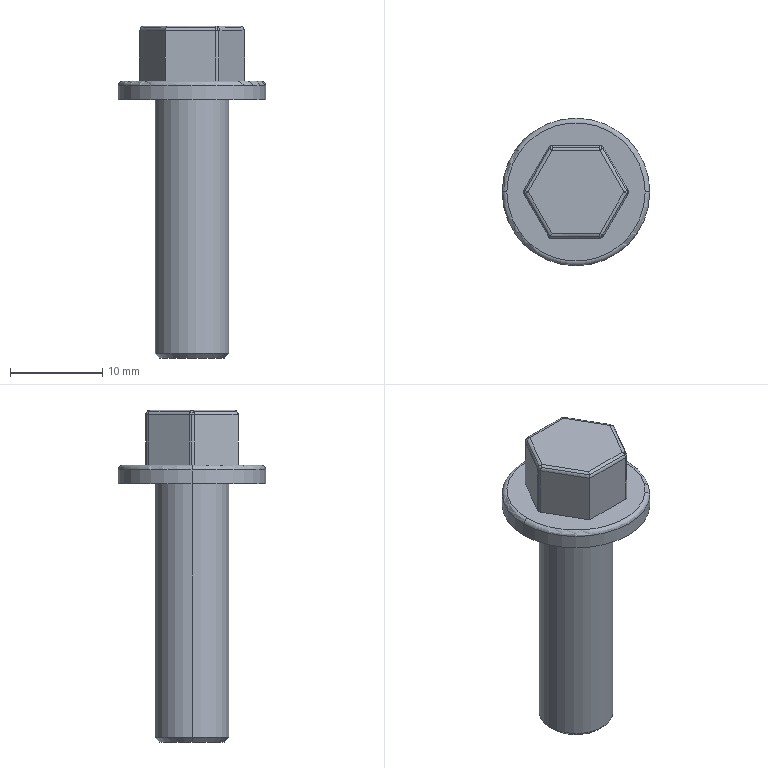Part | SolidWorks | features BaseBody 1 | 1 solid | 50 faces | box 16 x 16 x 36 mm | volume 2321 mm3 | cylinder 26 | sphere 10 | plane 10 | cone 2 | torus 2 | commonest cylinder face diameters 1 x22 8 x2 16 x2
STEP:
#1=CARTESIAN_POINT('',(3.5,0.,-28.));
#2=VERTEX_POINT('',#1);
#3=CARTESIAN_POINT('',(-3.5,0.,-28.));
#4=VERTEX_POINT('',#3);
#5=CARTESIAN_POINT('',(0.,0.,-28.));
#6=DIRECTION('',(0.,0.,1.));
#7=DIRECTION('',(1.,0.,0.));
#8=AXIS2_PLACEMENT_3D('',#5,#6,#7);
#9=CIRCLE('',#8,3.5);
#10=EDGE_CURVE('',#2,#4,#9,.T.);
#11=ORIENTED_EDGE('',*,*,#10,.T.);
#12=CARTESIAN_POINT('',(-4.,0.,-27.5));
#13=VERTEX_POINT('',#12);
#14=CARTESIAN_POINT('',(-3.75,0.,-27.75));
#15=DIRECTION('',(-0.7071,0.,0.7071));
#16=VECTOR('',#15,1000.);
#17=LINE('',#14,#16);
#18=EDGE_CURVE('',#4,#13,#17,.T.);
#19=ORIENTED_EDGE('',*,*,#18,.T.);
#20=CARTESIAN_POINT('',(4.,0.,-27.5));
#21=VERTEX_POINT('',#20);
#22=CARTESIAN_POINT('',(0.,0.,-27.5));
#23=DIRECTION('',(0.,0.,-1.));
#24=DIRECTION('',(1.,0.,0.));
#25=AXIS2_PLACEMENT_3D('',#22,#23,#24);
#26=CIRCLE('',#25,4.);
#27=EDGE_CURVE('',#13,#21,#26,.T.);
#28=ORIENTED_EDGE('',*,*,#27,.T.);
#29=CARTESIAN_POINT('',(3.75,0.,-27.75));
#30=DIRECTION('',(0.7071,0.,0.7071));
#31=VECTOR('',#30,1000.);
#32=LINE('',#29,#31);
#33=EDGE_CURVE('',#2,#21,#32,.T.);
#34=ORIENTED_EDGE('',*,*,#33,.F.);
#35=EDGE_LOOP('',(#11,#19,#28,#34));
#36=FACE_OUTER_BOUND('',#35,.T.);
#37=CARTESIAN_POINT('',(0.,0.,-27.75));
#38=DIRECTION('',(0.,0.,1.));
#39=DIRECTION('',(1.,0.,0.));
#40=AXIS2_PLACEMENT_3D('',#37,#38,#39);
#41=CONICAL_SURFACE('',#40,3.75,0.7854);
#42=ADVANCED_FACE('',(#36),#41,.T.);
#43=ORIENTED_EDGE('',*,*,#27,.F.);
#44=CARTESIAN_POINT('',(-4.,0.,0.));
#45=VERTEX_POINT('',#44);
#46=CARTESIAN_POINT('',(-4.,0.,0.));
#47=DIRECTION('',(0.,0.,1.));
#48=VECTOR('',#47,1000.);
#49=LINE('',#46,#48);
#50=EDGE_CURVE('',#13,#45,#49,.T.);
#51=ORIENTED_EDGE('',*,*,#50,.T.);
#52=CARTESIAN_POINT('',(4.,0.,0.));
#53=VERTEX_POINT('',#52);
#54=CARTESIAN_POINT('',(0.,0.,0.));
#55=DIRECTION('',(0.,0.,1.));
#56=DIRECTION('',(1.,0.,0.));
#57=AXIS2_PLACEMENT_3D('',#54,#55,#56);
#58=CIRCLE('',#57,4.);
#59=EDGE_CURVE('',#53,#45,#58,.T.);
#60=ORIENTED_EDGE('',*,*,#59,.F.);
#61=CARTESIAN_POINT('',(4.,0.,0.));
#62=DIRECTION('',(0.,0.,1.));
#63=VECTOR('',#62,1000.);
#64=LINE('',#61,#63);
#65=EDGE_CURVE('',#21,#53,#64,.T.);
#66=ORIENTED_EDGE('',*,*,#65,.F.);
#67=EDGE_LOOP('',(#43,#51,#60,#66));
#68=FACE_OUTER_BOUND('',#67,.T.);
#69=CARTESIAN_POINT('',(0.,0.,0.));
#70=DIRECTION('',(0.,0.,1.));
#71=DIRECTION('',(1.,0.,0.));
#72=AXIS2_PLACEMENT_3D('',#69,#70,#71);
#73=CYLINDRICAL_SURFACE('',#72,4.);
#74=ADVANCED_FACE('',(#68),#73,.T.);
#75=CARTESIAN_POINT('',(2.784,-4.964,7.5));
#76=VERTEX_POINT('',#75);
#77=CARTESIAN_POINT('',(2.598,-5.,7.5));
#78=VERTEX_POINT('',#77);
#79=CARTESIAN_POINT('',(2.598,-4.5,7.5));
#80=DIRECTION('',(0.,0.,-1.));
#81=DIRECTION('',(0.866,-0.5,0.));
#82=AXIS2_PLACEMENT_3D('',#79,#80,#81);
#83=CIRCLE('',#82,0.5);
#84=EDGE_CURVE('',#76,#78,#83,.T.);
#85=ORIENTED_EDGE('',*,*,#84,.F.);
#86=CARTESIAN_POINT('',(2.759,-4.593,7.964));
#87=VERTEX_POINT('',#86);
#88=CARTESIAN_POINT('',(2.598,-4.5,7.5));
#89=DIRECTION('',(-0.9014,-0.3603,0.2402));
#90=DIRECTION('',(0.3712,-0.9286,0.));
#91=AXIS2_PLACEMENT_3D('',#88,#89,#90);
#92=CIRCLE('',#91,0.5);
#93=EDGE_CURVE('',#76,#87,#92,.T.);
#94=ORIENTED_EDGE('',*,*,#93,.T.);
#95=CARTESIAN_POINT('',(2.598,-4.5,8.));
#96=VERTEX_POINT('',#95);
#97=CARTESIAN_POINT('',(2.598,-4.5,7.5));
#98=DIRECTION('',(0.5,0.866,0.));
#99=DIRECTION('',(0.,0.,1.));
#100=AXIS2_PLACEMENT_3D('',#97,#98,#99);
#101=CIRCLE('',#100,0.5);
#102=EDGE_CURVE('',#96,#87,#101,.T.);
#103=ORIENTED_EDGE('',*,*,#102,.F.);
#104=CARTESIAN_POINT('',(2.598,-4.854,7.854));
#105=VERTEX_POINT('',#104);
#106=CARTESIAN_POINT('',(2.598,-4.5,7.5));
#107=DIRECTION('',(-1.,0.,0.));
#108=DIRECTION('',(0.,-1.,0.));
#109=AXIS2_PLACEMENT_3D('',#106,#107,#108);
#110=CIRCLE('',#109,0.5);
#111=EDGE_CURVE('',#105,#96,#110,.T.);
#112=ORIENTED_EDGE('',*,*,#111,.F.);
#113=CARTESIAN_POINT('',(2.598,-4.5,7.5));
#114=DIRECTION('',(-1.,0.,0.));
#115=DIRECTION('',(0.,-1.,0.));
#116=AXIS2_PLACEMENT_3D('',#113,#114,#115);
#117=CIRCLE('',#116,0.5);
#118=EDGE_CURVE('',#78,#105,#117,.T.);
#119=ORIENTED_EDGE('',*,*,#118,.F.);
#120=EDGE_LOOP('',(#85,#94,#103,#112,#119));
#121=FACE_OUTER_BOUND('',#120,.T.);
#122=CARTESIAN_POINT('',(2.598,-4.5,7.5));
#123=DIRECTION('',(0.9014,0.3603,-0.2402));
#124=DIRECTION('',(0.433,-0.75,0.5));
#125=AXIS2_PLACEMENT_3D('',#122,#123,#124);
#126=SPHERICAL_SURFACE('',#125,0.5);
#127=ADVANCED_FACE('',(#121),#126,.T.);
#128=CARTESIAN_POINT('',(3.031,-4.75,7.5));
#129=VERTEX_POINT('',#128);
#130=CARTESIAN_POINT('',(2.848,-4.933,7.5));
#131=VERTEX_POINT('',#130);
#132=CARTESIAN_POINT('',(2.598,-4.5,7.5));
#133=DIRECTION('',(0.,0.,-1.));
#134=DIRECTION('',(0.866,-0.5,0.));
#135=AXIS2_PLACEMENT_3D('',#132,#133,#134);
#136=CIRCLE('',#135,0.5);
#137=EDGE_CURVE('',#129,#131,#136,.T.);
#138=ORIENTED_EDGE('',*,*,#137,.T.);
#139=CARTESIAN_POINT('',(2.848,-4.933,2.));
#140=VERTEX_POINT('',#139);
#141=CARTESIAN_POINT('',(2.848,-4.933,2.));
#142=DIRECTION('',(0.,0.,-1.));
#143=VECTOR('',#142,1000.);
#144=LINE('',#141,#143);
#145=EDGE_CURVE('',#131,#140,#144,.T.);
#146=ORIENTED_EDGE('',*,*,#145,.T.);
#147=CARTESIAN_POINT('',(3.031,-4.75,2.));
#148=VERTEX_POINT('',#147);
#149=CARTESIAN_POINT('',(2.598,-4.5,2.));
#150=DIRECTION('',(0.,0.,1.));
#151=DIRECTION('',(0.5,-0.866,0.));
#152=AXIS2_PLACEMENT_3D('',#149,#150,#151);
#153=CIRCLE('',#152,0.5);
#154=EDGE_CURVE('',#140,#148,#153,.T.);
#155=ORIENTED_EDGE('',*,*,#154,.T.);
#156=CARTESIAN_POINT('',(3.031,-4.75,2.));
#157=DIRECTION('',(0.,0.,1.));
#158=VECTOR('',#157,1000.);
#159=LINE('',#156,#158);
#160=EDGE_CURVE('',#148,#129,#159,.T.);
#161=ORIENTED_EDGE('',*,*,#160,.T.);
#162=EDGE_LOOP('',(#138,#146,#155,#161));
#163=FACE_OUTER_BOUND('',#162,.T.);
#164=CARTESIAN_POINT('',(2.598,-4.5,2.));
#165=DIRECTION('',(0.,0.,-1.));
#166=DIRECTION('',(0.5,-0.866,0.));
#167=AXIS2_PLACEMENT_3D('',#164,#165,#166);
#168=CYLINDRICAL_SURFACE('',#167,0.5);
#169=ADVANCED_FACE('',(#163),#168,.T.);
#170=ORIENTED_EDGE('',*,*,#118,.T.);
#171=CARTESIAN_POINT('',(-2.802,-4.854,7.854));
#172=VERTEX_POINT('',#171);
#173=CARTESIAN_POINT('',(-1.443,-4.854,7.854));
#174=DIRECTION('',(-1.,0.,0.));
#175=VECTOR('',#174,1000.);
#176=LINE('',#173,#175);
#177=EDGE_CURVE('',#105,#172,#176,.T.);
#178=ORIENTED_EDGE('',*,*,#177,.T.);
#179=CARTESIAN_POINT('',(-2.887,-5.,7.5));
#180=VERTEX_POINT('',#179);
#181=CARTESIAN_POINT('',(-2.802,-4.854,7.854));
#182=CARTESIAN_POINT('',(-2.857,-4.949,7.759));
#183=CARTESIAN_POINT('',(-2.887,-5.,7.634));
#184=CARTESIAN_POINT('',(-2.887,-5.,7.5));
#185=(BOUNDED_CURVE()B_SPLINE_CURVE(3,(#181,#182,#183,#184),.UNSPECIFIED.,.F.,.F.)B_SPLINE_CURVE_WITH_KNOTS((4,4),(5.498,6.283),.UNSPECIFIED.)CURVE()GEOMETRIC_REPRESENTATION_ITEM()RATIONAL_B_SPLINE_CURVE((1.,0.9493,0.9493,1.))REPRESENTATION_ITEM(''));
#186=EDGE_CURVE('',#172,#180,#185,.T.);
#187=ORIENTED_EDGE('',*,*,#186,.T.);
#188=CARTESIAN_POINT('',(-1.443,-5.,7.5));
#189=DIRECTION('',(1.,0.,0.));
#190=VECTOR('',#189,1000.);
#191=LINE('',#188,#190);
#192=EDGE_CURVE('',#180,#78,#191,.T.);
#193=ORIENTED_EDGE('',*,*,#192,.T.);
#194=EDGE_LOOP('',(#170,#178,#187,#193));
#195=FACE_OUTER_BOUND('',#194,.T.);
#196=CARTESIAN_POINT('',(-1.443,-4.5,7.5));
#197=DIRECTION('',(-1.,0.,0.));
#198=DIRECTION('',(0.,-0.7071,0.7071));
#199=AXIS2_PLACEMENT_3D('',#196,#197,#198);
#200=CYLINDRICAL_SURFACE('',#199,0.5);
#201=ADVANCED_FACE('',(#195),#200,.T.);
#202=CARTESIAN_POINT('',(-5.583,-0.2236,7.724));
#203=VERTEX_POINT('',#202);
#204=CARTESIAN_POINT('',(-5.629,-0.25,7.5));
#205=VERTEX_POINT('',#204);
#206=CARTESIAN_POINT('',(-5.196,0.,7.5));
#207=DIRECTION('',(0.5,-0.866,0.));
#208=DIRECTION('',(0.,0.,1.));
#209=AXIS2_PLACEMENT_3D('',#206,#207,#208);
#210=CIRCLE('',#209,0.5);
#211=EDGE_CURVE('',#203,#205,#210,.T.);
#212=ORIENTED_EDGE('',*,*,#211,.F.);
#213=CARTESIAN_POINT('',(-5.583,0.2236,7.724));
#214=VERTEX_POINT('',#213);
#215=CARTESIAN_POINT('',(-5.196,0.,7.5));
#216=DIRECTION('',(-0.5,0.,-0.866));
#217=DIRECTION('',(-0.866,0.,0.5));
#218=AXIS2_PLACEMENT_3D('',#215,#216,#217);
#219=CIRCLE('',#218,0.5);
#220=EDGE_CURVE('',#203,#214,#219,.T.);
#221=ORIENTED_EDGE('',*,*,#220,.T.);
#222=CARTESIAN_POINT('',(-5.629,0.25,7.5));
#223=VERTEX_POINT('',#222);
#224=CARTESIAN_POINT('',(-5.196,0.,7.5));
#225=DIRECTION('',(0.5,0.866,0.));
#226=DIRECTION('',(-0.866,0.5,0.));
#227=AXIS2_PLACEMENT_3D('',#224,#225,#226);
#228=CIRCLE('',#227,0.5);
#229=EDGE_CURVE('',#223,#214,#228,.T.);
#230=ORIENTED_EDGE('',*,*,#229,.F.);
#231=CARTESIAN_POINT('',(-5.696,0.,7.5));
#232=VERTEX_POINT('',#231);
#233=CARTESIAN_POINT('',(-5.196,0.,7.5));
#234=DIRECTION('',(0.,0.,-1.));
#235=DIRECTION('',(-0.866,-0.5,0.));
#236=AXIS2_PLACEMENT_3D('',#233,#234,#235);
#237=CIRCLE('',#236,0.5);
#238=EDGE_CURVE('',#232,#223,#237,.T.);
#239=ORIENTED_EDGE('',*,*,#238,.F.);
#240=CARTESIAN_POINT('',(-5.196,0.,7.5));
#241=DIRECTION('',(0.,0.,-1.));
#242=DIRECTION('',(-0.866,-0.5,0.));
#243=AXIS2_PLACEMENT_3D('',#240,#241,#242);
#244=CIRCLE('',#243,0.5);
#245=EDGE_CURVE('',#205,#232,#244,.T.);
#246=ORIENTED_EDGE('',*,*,#245,.F.);
#247=EDGE_LOOP('',(#212,#221,#230,#239,#246));
#248=FACE_OUTER_BOUND('',#247,.T.);
#249=CARTESIAN_POINT('',(-5.196,0.,7.5));
#250=DIRECTION('',(0.5,0.,0.866));
#251=DIRECTION('',(-0.866,0.,0.5));
#252=AXIS2_PLACEMENT_3D('',#249,#250,#251);
#253=SPHERICAL_SURFACE('',#252,0.5);
#254=ADVANCED_FACE('',(#248),#253,.T.);
#255=ORIENTED_EDGE('',*,*,#245,.T.);
#256=CARTESIAN_POINT('',(-5.696,0.,2.));
#257=VERTEX_POINT('',#256);
#258=CARTESIAN_POINT('',(-5.696,0.,2.));
#259=DIRECTION('',(0.,0.,-1.));
#260=VECTOR('',#259,1000.);
#261=LINE('',#258,#260);
#262=EDGE_CURVE('',#232,#257,#261,.T.);
#263=ORIENTED_EDGE('',*,*,#262,.T.);
#264=CARTESIAN_POINT('',(-5.629,-0.25,2.));
#265=VERTEX_POINT('',#264);
#266=CARTESIAN_POINT('',(-5.196,0.,2.));
#267=DIRECTION('',(0.,0.,1.));
#268=DIRECTION('',(-1.,0.,0.));
#269=AXIS2_PLACEMENT_3D('',#266,#267,#268);
#270=CIRCLE('',#269,0.5);
#271=EDGE_CURVE('',#257,#265,#270,.T.);
#272=ORIENTED_EDGE('',*,*,#271,.T.);
#273=CARTESIAN_POINT('',(-5.629,-0.25,2.));
#274=DIRECTION('',(0.,0.,1.));
#275=VECTOR('',#274,1000.);
#276=LINE('',#273,#275);
#277=EDGE_CURVE('',#265,#205,#276,.T.);
#278=ORIENTED_EDGE('',*,*,#277,.T.);
#279=EDGE_LOOP('',(#255,#263,#272,#278));
#280=FACE_OUTER_BOUND('',#279,.T.);
#281=CARTESIAN_POINT('',(-5.196,0.,2.));
#282=DIRECTION('',(0.,0.,-1.));
#283=DIRECTION('',(-1.,0.,0.));
#284=AXIS2_PLACEMENT_3D('',#281,#282,#283);
#285=CYLINDRICAL_SURFACE('',#284,0.5);
#286=ADVANCED_FACE('',(#280),#285,.T.);
#287=ORIENTED_EDGE('',*,*,#186,.F.);
#288=CARTESIAN_POINT('',(-5.502,-0.1768,7.854));
#289=VERTEX_POINT('',#288);
#290=CARTESIAN_POINT('',(-4.925,-1.177,7.854));
#291=DIRECTION('',(-0.5,0.866,0.));
#292=VECTOR('',#291,1000.);
#293=LINE('',#290,#292);
#294=EDGE_CURVE('',#172,#289,#293,.T.);
#295=ORIENTED_EDGE('',*,*,#294,.T.);
#296=CARTESIAN_POINT('',(-5.196,0.,7.5));
#297=DIRECTION('',(0.5,-0.866,0.));
#298=DIRECTION('',(0.,0.,1.));
#299=AXIS2_PLACEMENT_3D('',#296,#297,#298);
#300=CIRCLE('',#299,0.5);
#301=EDGE_CURVE('',#289,#203,#300,.T.);
#302=ORIENTED_EDGE('',*,*,#301,.T.);
#303=ORIENTED_EDGE('',*,*,#211,.T.);
#304=CARTESIAN_POINT('',(-5.052,-1.25,7.5));
#305=DIRECTION('',(0.5,-0.866,0.));
#306=VECTOR('',#305,1000.);
#307=LINE('',#304,#306);
#308=EDGE_CURVE('',#205,#180,#307,.T.);
#309=ORIENTED_EDGE('',*,*,#308,.T.);
#310=EDGE_LOOP('',(#287,#295,#302,#303,#309));
#311=FACE_OUTER_BOUND('',#310,.T.);
#312=CARTESIAN_POINT('',(-4.619,-1.,7.5));
#313=DIRECTION('',(-0.5,0.866,0.));
#314=DIRECTION('',(-0.6124,-0.3536,0.7071));
#315=AXIS2_PLACEMENT_3D('',#312,#313,#314);
#316=CYLINDRICAL_SURFACE('',#315,0.5);
#317=ADVANCED_FACE('',(#311),#316,.T.);
#318=CARTESIAN_POINT('',(5.583,0.2236,7.724));
#319=VERTEX_POINT('',#318);
#320=CARTESIAN_POINT('',(5.629,0.25,7.5));
#321=VERTEX_POINT('',#320);
#322=CARTESIAN_POINT('',(5.196,0.,7.5));
#323=DIRECTION('',(-0.5,0.866,0.));
#324=DIRECTION('',(0.,0.,1.));
#325=AXIS2_PLACEMENT_3D('',#322,#323,#324);
#326=CIRCLE('',#325,0.5);
#327=EDGE_CURVE('',#319,#321,#326,.T.);
#328=ORIENTED_EDGE('',*,*,#327,.F.);
#329=CARTESIAN_POINT('',(5.583,-0.2236,7.724));
#330=VERTEX_POINT('',#329);
#331=CARTESIAN_POINT('',(5.196,0.,7.5));
#332=DIRECTION('',(0.5,0.,-0.866));
#333=DIRECTION('',(-0.866,0.,-0.5));
#334=AXIS2_PLACEMENT_3D('',#331,#332,#333);
#335=CIRCLE('',#334,0.5);
#336=EDGE_CURVE('',#319,#330,#335,.T.);
#337=ORIENTED_EDGE('',*,*,#336,.T.);
#338=CARTESIAN_POINT('',(5.629,-0.25,7.5));
#339=VERTEX_POINT('',#338);
#340=CARTESIAN_POINT('',(5.196,0.,7.5));
#341=DIRECTION('',(-0.5,-0.866,0.));
#342=DIRECTION('',(0.866,-0.5,0.));
#343=AXIS2_PLACEMENT_3D('',#340,#341,#342);
#344=CIRCLE('',#343,0.5);
#345=EDGE_CURVE('',#339,#330,#344,.T.);
#346=ORIENTED_EDGE('',*,*,#345,.F.);
#347=CARTESIAN_POINT('',(5.696,0.,7.5));
#348=VERTEX_POINT('',#347);
#349=CARTESIAN_POINT('',(5.196,0.,7.5));
#350=DIRECTION('',(0.,0.,-1.));
#351=DIRECTION('',(0.866,0.5,0.));
#352=AXIS2_PLACEMENT_3D('',#349,#350,#351);
#353=CIRCLE('',#352,0.5);
#354=EDGE_CURVE('',#348,#339,#353,.T.);
#355=ORIENTED_EDGE('',*,*,#354,.F.);
#356=CARTESIAN_POINT('',(5.196,0.,7.5));
#357=DIRECTION('',(0.,0.,-1.));
#358=DIRECTION('',(0.866,0.5,0.));
#359=AXIS2_PLACEMENT_3D('',#356,#357,#358);
#360=CIRCLE('',#359,0.5);
#361=EDGE_CURVE('',#321,#348,#360,.T.);
#362=ORIENTED_EDGE('',*,*,#361,.F.);
#363=EDGE_LOOP('',(#328,#337,#346,#355,#362));
#364=FACE_OUTER_BOUND('',#363,.T.);
#365=CARTESIAN_POINT('',(5.196,0.,7.5));
#366=DIRECTION('',(-0.5,0.,0.866));
#367=DIRECTION('',(0.866,0.,0.5));
#368=AXIS2_PLACEMENT_3D('',#365,#366,#367);
#369=SPHERICAL_SURFACE('',#368,0.5);
#370=ADVANCED_FACE('',(#364),#369,.T.);
#371=ORIENTED_EDGE('',*,*,#361,.T.);
#372=CARTESIAN_POINT('',(5.696,0.,2.));
#373=VERTEX_POINT('',#372);
#374=CARTESIAN_POINT('',(5.696,0.,2.));
#375=DIRECTION('',(0.,0.,-1.));
#376=VECTOR('',#375,1000.);
#377=LINE('',#374,#376);
#378=EDGE_CURVE('',#348,#373,#377,.T.);
#379=ORIENTED_EDGE('',*,*,#378,.T.);
#380=CARTESIAN_POINT('',(5.629,0.25,2.));
#381=VERTEX_POINT('',#380);
#382=CARTESIAN_POINT('',(5.196,0.,2.));
#383=DIRECTION('',(0.,0.,1.));
#384=DIRECTION('',(1.,0.,0.));
#385=AXIS2_PLACEMENT_3D('',#382,#383,#384);
#386=CIRCLE('',#385,0.5);
#387=EDGE_CURVE('',#373,#381,#386,.T.);
#388=ORIENTED_EDGE('',*,*,#387,.T.);
#389=CARTESIAN_POINT('',(5.629,0.25,2.));
#390=DIRECTION('',(0.,0.,1.));
#391=VECTOR('',#390,1000.);
#392=LINE('',#389,#391);
#393=EDGE_CURVE('',#381,#321,#392,.T.);
#394=ORIENTED_EDGE('',*,*,#393,.T.);
#395=EDGE_LOOP('',(#371,#379,#388,#394));
#396=FACE_OUTER_BOUND('',#395,.T.);
#397=CARTESIAN_POINT('',(5.196,0.,2.));
#398=DIRECTION('',(0.,0.,-1.));
#399=DIRECTION('',(1.,0.,0.));
#400=AXIS2_PLACEMENT_3D('',#397,#398,#399);
#401=CYLINDRICAL_SURFACE('',#400,0.5);
#402=ADVANCED_FACE('',(#396),#401,.T.);
#403=CARTESIAN_POINT('',(-2.759,4.593,7.964));
#404=VERTEX_POINT('',#403);
#405=CARTESIAN_POINT('',(-2.904,4.677,7.854));
#406=VERTEX_POINT('',#405);
#407=CARTESIAN_POINT('',(-2.598,4.5,7.5));
#408=DIRECTION('',(-0.5,-0.866,0.));
#409=DIRECTION('',(0.,0.,1.));
#410=AXIS2_PLACEMENT_3D('',#407,#408,#409);
#411=CIRCLE('',#410,0.5);
#412=EDGE_CURVE('',#404,#406,#411,.T.);
#413=ORIENTED_EDGE('',*,*,#412,.F.);
#414=CARTESIAN_POINT('',(-2.784,4.964,7.5));
#415=VERTEX_POINT('',#414);
#416=CARTESIAN_POINT('',(-2.598,4.5,7.5));
#417=DIRECTION('',(-0.9014,-0.3603,-0.2402));
#418=DIRECTION('',(0.3712,-0.9286,0.));
#419=AXIS2_PLACEMENT_3D('',#416,#417,#418);
#420=CIRCLE('',#419,0.5);
#421=EDGE_CURVE('',#404,#415,#420,.T.);
#422=ORIENTED_EDGE('',*,*,#421,.T.);
#423=CARTESIAN_POINT('',(-2.848,4.933,7.5));
#424=VERTEX_POINT('',#423);
#425=CARTESIAN_POINT('',(-2.598,4.5,7.5));
#426=DIRECTION('',(0.,0.,-1.));
#427=DIRECTION('',(-0.866,0.5,0.));
#428=AXIS2_PLACEMENT_3D('',#425,#426,#427);
#429=CIRCLE('',#428,0.5);
#430=EDGE_CURVE('',#424,#415,#429,.T.);
#431=ORIENTED_EDGE('',*,*,#430,.F.);
#432=CARTESIAN_POINT('',(-3.031,4.75,7.5));
#433=VERTEX_POINT('',#432);
#434=CARTESIAN_POINT('',(-2.598,4.5,7.5));
#435=DIRECTION('',(0.,0.,-1.));
#436=DIRECTION('',(-0.866,0.5,0.));
#437=AXIS2_PLACEMENT_3D('',#434,#435,#436);
#438=CIRCLE('',#437,0.5);
#439=EDGE_CURVE('',#433,#424,#438,.T.);
#440=ORIENTED_EDGE('',*,*,#439,.F.);
#441=CARTESIAN_POINT('',(-2.598,4.5,7.5));
#442=DIRECTION('',(-0.5,-0.866,0.));
#443=DIRECTION('',(0.,0.,1.));
#444=AXIS2_PLACEMENT_3D('',#441,#442,#443);
#445=CIRCLE('',#444,0.5);
#446=EDGE_CURVE('',#406,#433,#445,.T.);
#447=ORIENTED_EDGE('',*,*,#446,.F.);
#448=EDGE_LOOP('',(#413,#422,#431,#440,#447));
#449=FACE_OUTER_BOUND('',#448,.T.);
#450=CARTESIAN_POINT('',(-2.598,4.5,7.5));
#451=DIRECTION('',(0.9014,0.3603,0.2402));
#452=DIRECTION('',(-0.433,0.75,0.5));
#453=AXIS2_PLACEMENT_3D('',#450,#451,#452);
#454=SPHERICAL_SURFACE('',#453,0.5);
#455=ADVANCED_FACE('',(#449),#454,.T.);
#456=ORIENTED_EDGE('',*,*,#439,.T.);
#457=CARTESIAN_POINT('',(-2.848,4.933,2.));
#458=VERTEX_POINT('',#457);
#459=CARTESIAN_POINT('',(-2.848,4.933,2.));
#460=DIRECTION('',(0.,0.,-1.));
#461=VECTOR('',#460,1000.);
#462=LINE('',#459,#461);
#463=EDGE_CURVE('',#424,#458,#462,.T.);
#464=ORIENTED_EDGE('',*,*,#463,.T.);
#465=CARTESIAN_POINT('',(-3.031,4.75,2.));
#466=VERTEX_POINT('',#465);
#467=CARTESIAN_POINT('',(-2.598,4.5,2.));
#468=DIRECTION('',(0.,0.,1.));
#469=DIRECTION('',(-0.5,0.866,0.));
#470=AXIS2_PLACEMENT_3D('',#467,#468,#469);
#471=CIRCLE('',#470,0.5);
#472=EDGE_CURVE('',#458,#466,#471,.T.);
#473=ORIENTED_EDGE('',*,*,#472,.T.);
#474=CARTESIAN_POINT('',(-3.031,4.75,2.));
#475=DIRECTION('',(0.,0.,1.));
#476=VECTOR('',#475,1000.);
#477=LINE('',#474,#476);
#478=EDGE_CURVE('',#466,#433,#477,.T.);
#479=ORIENTED_EDGE('',*,*,#478,.T.);
#480=EDGE_LOOP('',(#456,#464,#473,#479));
#481=FACE_OUTER_BOUND('',#480,.T.);
#482=CARTESIAN_POINT('',(-2.598,4.5,2.));
#483=DIRECTION('',(0.,0.,-1.));
#484=DIRECTION('',(-0.5,0.866,0.));
#485=AXIS2_PLACEMENT_3D('',#482,#483,#484);
#486=CYLINDRICAL_SURFACE('',#485,0.5);
#487=ADVANCED_FACE('',(#481),#486,.T.);
#488=ORIENTED_EDGE('',*,*,#229,.T.);
#489=CARTESIAN_POINT('',(-5.502,0.1768,7.854));
#490=VERTEX_POINT('',#489);
#491=CARTESIAN_POINT('',(-5.196,0.,7.5));
#492=DIRECTION('',(0.5,0.866,0.));
#493=DIRECTION('',(-0.866,0.5,0.));
#494=AXIS2_PLACEMENT_3D('',#491,#492,#493);
#495=CIRCLE('',#494,0.5);
#496=EDGE_CURVE('',#214,#490,#495,.T.);
#497=ORIENTED_EDGE('',*,*,#496,.T.);
#498=CARTESIAN_POINT('',(-3.482,3.677,7.854));
#499=DIRECTION('',(0.5,0.866,0.));
#500=VECTOR('',#499,1000.);
#501=LINE('',#498,#500);
#502=EDGE_CURVE('',#490,#406,#501,.T.);
#503=ORIENTED_EDGE('',*,*,#502,.T.);
#504=ORIENTED_EDGE('',*,*,#446,.T.);
#505=CARTESIAN_POINT('',(-3.608,3.75,7.5));
#506=DIRECTION('',(-0.5,-0.866,0.));
#507=VECTOR('',#506,1000.);
#508=LINE('',#505,#507);
#509=EDGE_CURVE('',#433,#223,#508,.T.);
#510=ORIENTED_EDGE('',*,*,#509,.T.);
#511=EDGE_LOOP('',(#488,#497,#503,#504,#510));
#512=FACE_OUTER_BOUND('',#511,.T.);
#513=CARTESIAN_POINT('',(-3.175,3.5,7.5));
#514=DIRECTION('',(0.5,0.866,0.));
#515=DIRECTION('',(-0.6124,0.3536,0.7071));
#516=AXIS2_PLACEMENT_3D('',#513,#514,#515);
#517=CYLINDRICAL_SURFACE('',#516,0.5);
#518=ADVANCED_FACE('',(#512),#517,.T.);
#519=CARTESIAN_POINT('',(2.759,4.593,7.964));
#520=VERTEX_POINT('',#519);
#521=CARTESIAN_POINT('',(2.598,4.5,8.));
#522=VERTEX_POINT('',#521);
#523=CARTESIAN_POINT('',(2.598,4.5,7.5));
#524=DIRECTION('',(0.5,-0.866,0.));
#525=DIRECTION('',(0.866,0.5,0.));
#526=AXIS2_PLACEMENT_3D('',#523,#524,#525);
#527=CIRCLE('',#526,0.5);
#528=EDGE_CURVE('',#520,#522,#527,.T.);
#529=ORIENTED_EDGE('',*,*,#528,.F.);
#530=CARTESIAN_POINT('',(2.784,4.964,7.5));
#531=VERTEX_POINT('',#530);
#532=CARTESIAN_POINT('',(2.598,4.5,7.5));
#533=DIRECTION('',(-0.9014,0.3603,0.2402));
#534=DIRECTION('',(-0.3712,-0.9286,0.));
#535=AXIS2_PLACEMENT_3D('',#532,#533,#534);
#536=CIRCLE('',#535,0.5);
#537=EDGE_CURVE('',#520,#531,#536,.T.);
#538=ORIENTED_EDGE('',*,*,#537,.T.);
#539=CARTESIAN_POINT('',(2.598,5.,7.5));
#540=VERTEX_POINT('',#539);
#541=CARTESIAN_POINT('',(2.598,4.5,7.5));
#542=DIRECTION('',(0.,0.,-1.));
#543=DIRECTION('',(0.,1.,0.));
#544=AXIS2_PLACEMENT_3D('',#541,#542,#543);
#545=CIRCLE('',#544,0.5);
#546=EDGE_CURVE('',#540,#531,#545,.T.);
#547=ORIENTED_EDGE('',*,*,#546,.F.);
#548=CARTESIAN_POINT('',(2.598,4.854,7.854));
#549=VERTEX_POINT('',#548);
#550=CARTESIAN_POINT('',(2.598,4.5,7.5));
#551=DIRECTION('',(-1.,0.,0.));
#552=DIRECTION('',(0.,0.,1.));
#553=AXIS2_PLACEMENT_3D('',#550,#551,#552);
#554=CIRCLE('',#553,0.5);
#555=EDGE_CURVE('',#549,#540,#554,.T.);
#556=ORIENTED_EDGE('',*,*,#555,.F.);
#557=CARTESIAN_POINT('',(2.598,4.5,7.5));
#558=DIRECTION('',(-1.,0.,0.));
#559=DIRECTION('',(0.,0.,1.));
#560=AXIS2_PLACEMENT_3D('',#557,#558,#559);
#561=CIRCLE('',#560,0.5);
#562=EDGE_CURVE('',#522,#549,#561,.T.);
#563=ORIENTED_EDGE('',*,*,#562,.F.);
#564=EDGE_LOOP('',(#529,#538,#547,#556,#563));
#565=FACE_OUTER_BOUND('',#564,.T.);
#566=CARTESIAN_POINT('',(2.598,4.5,7.5));
#567=DIRECTION('',(0.9014,-0.3603,-0.2402));
#568=DIRECTION('',(0.433,0.75,0.5));
#569=AXIS2_PLACEMENT_3D('',#566,#567,#568);
#570=SPHERICAL_SURFACE('',#569,0.5);
#571=ADVANCED_FACE('',(#565),#570,.T.);
#572=ORIENTED_EDGE('',*,*,#546,.T.);
#573=CARTESIAN_POINT('',(2.848,4.933,7.5));
#574=VERTEX_POINT('',#573);
#575=CARTESIAN_POINT('',(2.598,4.5,7.5));
#576=DIRECTION('',(0.,0.,-1.));
#577=DIRECTION('',(0.,1.,0.));
#578=AXIS2_PLACEMENT_3D('',#575,#576,#577);
#579=CIRCLE('',#578,0.5);
#580=EDGE_CURVE('',#531,#574,#579,.T.);
#581=ORIENTED_EDGE('',*,*,#580,.T.);
#582=CARTESIAN_POINT('',(2.848,4.933,2.));
#583=VERTEX_POINT('',#582);
#584=CARTESIAN_POINT('',(2.848,4.933,2.));
#585=DIRECTION('',(0.,0.,-1.));
#586=VECTOR('',#585,1000.);
#587=LINE('',#584,#586);
#588=EDGE_CURVE('',#574,#583,#587,.T.);
#589=ORIENTED_EDGE('',*,*,#588,.T.);
#590=CARTESIAN_POINT('',(2.598,5.,2.));
#591=VERTEX_POINT('',#590);
#592=CARTESIAN_POINT('',(2.598,4.5,2.));
#593=DIRECTION('',(0.,0.,1.));
#594=DIRECTION('',(0.5,0.866,0.));
#595=AXIS2_PLACEMENT_3D('',#592,#593,#594);
#596=CIRCLE('',#595,0.5);
#597=EDGE_CURVE('',#583,#591,#596,.T.);
#598=ORIENTED_EDGE('',*,*,#597,.T.);
#599=CARTESIAN_POINT('',(2.598,5.,2.));
#600=DIRECTION('',(0.,0.,1.));
#601=VECTOR('',#600,1000.);
#602=LINE('',#599,#601);
#603=EDGE_CURVE('',#591,#540,#602,.T.);
#604=ORIENTED_EDGE('',*,*,#603,.T.);
#605=EDGE_LOOP('',(#572,#581,#589,#598,#604));
#606=FACE_OUTER_BOUND('',#605,.T.);
#607=CARTESIAN_POINT('',(2.598,4.5,2.));
#608=DIRECTION('',(0.,0.,-1.));
#609=DIRECTION('',(0.5,0.866,0.));
#610=AXIS2_PLACEMENT_3D('',#607,#608,#609);
#611=CYLINDRICAL_SURFACE('',#610,0.5);
#612=ADVANCED_FACE('',(#606),#611,.T.);
#613=CARTESIAN_POINT('',(-2.598,5.,7.5));
#614=VERTEX_POINT('',#613);
#615=CARTESIAN_POINT('',(-2.598,4.854,7.854));
#616=VERTEX_POINT('',#615);
#617=CARTESIAN_POINT('',(-2.598,4.5,7.5));
#618=DIRECTION('',(1.,0.,0.));
#619=DIRECTION('',(0.,1.,0.));
#620=AXIS2_PLACEMENT_3D('',#617,#618,#619);
#621=CIRCLE('',#620,0.5);
#622=EDGE_CURVE('',#614,#616,#621,.T.);
#623=ORIENTED_EDGE('',*,*,#622,.T.);
#624=CARTESIAN_POINT('',(1.443,4.854,7.854));
#625=DIRECTION('',(1.,0.,0.));
#626=VECTOR('',#625,1000.);
#627=LINE('',#624,#626);
#628=EDGE_CURVE('',#616,#549,#627,.T.);
#629=ORIENTED_EDGE('',*,*,#628,.T.);
#630=ORIENTED_EDGE('',*,*,#555,.T.);
#631=CARTESIAN_POINT('',(1.443,5.,7.5));
#632=DIRECTION('',(-1.,0.,0.));
#633=VECTOR('',#632,1000.);
#634=LINE('',#631,#633);
#635=EDGE_CURVE('',#540,#614,#634,.T.);
#636=ORIENTED_EDGE('',*,*,#635,.T.);
#637=EDGE_LOOP('',(#623,#629,#630,#636));
#638=FACE_OUTER_BOUND('',#637,.T.);
#639=CARTESIAN_POINT('',(1.443,4.5,7.5));
#640=DIRECTION('',(1.,0.,0.));
#641=DIRECTION('',(0.,0.7071,0.7071));
#642=AXIS2_PLACEMENT_3D('',#639,#640,#641);
#643=CYLINDRICAL_SURFACE('',#642,0.5);
#644=ADVANCED_FACE('',(#638),#643,.T.);
#645=CARTESIAN_POINT('',(3.031,4.75,7.5));
#646=VERTEX_POINT('',#645);
#647=CARTESIAN_POINT('',(2.904,4.677,7.854));
#648=VERTEX_POINT('',#647);
#649=CARTESIAN_POINT('',(2.598,4.5,7.5));
#650=DIRECTION('',(0.5,-0.866,0.));
#651=DIRECTION('',(0.866,0.5,0.));
#652=AXIS2_PLACEMENT_3D('',#649,#650,#651);
#653=CIRCLE('',#652,0.5);
#654=EDGE_CURVE('',#646,#648,#653,.T.);
#655=ORIENTED_EDGE('',*,*,#654,.T.);
#656=CARTESIAN_POINT('',(5.502,0.1768,7.854));
#657=VERTEX_POINT('',#656);
#658=CARTESIAN_POINT('',(4.925,1.177,7.854));
#659=DIRECTION('',(0.5,-0.866,0.));
#660=VECTOR('',#659,1000.);
#661=LINE('',#658,#660);
#662=EDGE_CURVE('',#648,#657,#661,.T.);
#663=ORIENTED_EDGE('',*,*,#662,.T.);
#664=CARTESIAN_POINT('',(5.196,0.,7.5));
#665=DIRECTION('',(-0.5,0.866,0.));
#666=DIRECTION('',(0.,0.,1.));
#667=AXIS2_PLACEMENT_3D('',#664,#665,#666);
#668=CIRCLE('',#667,0.5);
#669=EDGE_CURVE('',#657,#319,#668,.T.);
#670=ORIENTED_EDGE('',*,*,#669,.T.);
#671=ORIENTED_EDGE('',*,*,#327,.T.);
#672=CARTESIAN_POINT('',(5.052,1.25,7.5));
#673=DIRECTION('',(-0.5,0.866,0.));
#674=VECTOR('',#673,1000.);
#675=LINE('',#672,#674);
#676=EDGE_CURVE('',#321,#646,#675,.T.);
#677=ORIENTED_EDGE('',*,*,#676,.T.);
#678=EDGE_LOOP('',(#655,#663,#670,#671,#677));
#679=FACE_OUTER_BOUND('',#678,.T.);
#680=CARTESIAN_POINT('',(4.619,1.,7.5));
#681=DIRECTION('',(0.5,-0.866,0.));
#682=DIRECTION('',(0.6124,0.3536,0.7071));
#683=AXIS2_PLACEMENT_3D('',#680,#681,#682);
#684=CYLINDRICAL_SURFACE('',#683,0.5);
#685=ADVANCED_FACE('',(#679),#684,.T.);
#686=ORIENTED_EDGE('',*,*,#345,.T.);
#687=CARTESIAN_POINT('',(5.502,-0.1768,7.854));
#688=VERTEX_POINT('',#687);
#689=CARTESIAN_POINT('',(5.196,0.,7.5));
#690=DIRECTION('',(-0.5,-0.866,0.));
#691=DIRECTION('',(0.866,-0.5,0.));
#692=AXIS2_PLACEMENT_3D('',#689,#690,#691);
#693=CIRCLE('',#692,0.5);
#694=EDGE_CURVE('',#330,#688,#693,.T.);
#695=ORIENTED_EDGE('',*,*,#694,.T.);
#696=CARTESIAN_POINT('',(2.904,-4.677,7.854));
#697=VERTEX_POINT('',#696);
#698=CARTESIAN_POINT('',(3.482,-3.677,7.854));
#699=DIRECTION('',(-0.5,-0.866,0.));
#700=VECTOR('',#699,1000.);
#701=LINE('',#698,#700);
#702=EDGE_CURVE('',#688,#697,#701,.T.);
#703=ORIENTED_EDGE('',*,*,#702,.T.);
#704=CARTESIAN_POINT('',(2.598,-4.5,7.5));
#705=DIRECTION('',(0.5,0.866,0.));
#706=DIRECTION('',(0.,0.,1.));
#707=AXIS2_PLACEMENT_3D('',#704,#705,#706);
#708=CIRCLE('',#707,0.5);
#709=EDGE_CURVE('',#697,#129,#708,.T.);
#710=ORIENTED_EDGE('',*,*,#709,.T.);
#711=CARTESIAN_POINT('',(3.608,-3.75,7.5));
#712=DIRECTION('',(0.5,0.866,0.));
#713=VECTOR('',#712,1000.);
#714=LINE('',#711,#713);
#715=EDGE_CURVE('',#129,#339,#714,.T.);
#716=ORIENTED_EDGE('',*,*,#715,.T.);
#717=EDGE_LOOP('',(#686,#695,#703,#710,#716));
#718=FACE_OUTER_BOUND('',#717,.T.);
#719=CARTESIAN_POINT('',(3.175,-3.5,7.5));
#720=DIRECTION('',(-0.5,-0.866,0.));
#721=DIRECTION('',(0.6124,-0.3536,0.7071));
#722=AXIS2_PLACEMENT_3D('',#719,#720,#721);
#723=CYLINDRICAL_SURFACE('',#722,0.5);
#724=ADVANCED_FACE('',(#718),#723,.T.);
#725=CARTESIAN_POINT('',(8.,0.,1.5));
#726=VERTEX_POINT('',#725);
#727=CARTESIAN_POINT('',(-8.,0.,1.5));
#728=VERTEX_POINT('',#727);
#729=CARTESIAN_POINT('',(0.,0.,1.5));
#730=DIRECTION('',(0.,0.,1.));
#731=DIRECTION('',(-1.,0.,0.));
#732=AXIS2_PLACEMENT_3D('',#729,#730,#731);
#733=CIRCLE('',#732,8.);
#734=EDGE_CURVE('',#726,#728,#733,.T.);
#735=ORIENTED_EDGE('',*,*,#734,.T.);
#736=CARTESIAN_POINT('',(-7.5,0.,2.));
#737=VERTEX_POINT('',#736);
#738=CARTESIAN_POINT('',(-7.5,0.,1.5));
#739=DIRECTION('',(0.,1.,0.));
#740=DIRECTION('',(-1.,0.,0.));
#741=AXIS2_PLACEMENT_3D('',#738,#739,#740);
#742=CIRCLE('',#741,0.5);
#743=EDGE_CURVE('',#728,#737,#742,.T.);
#744=ORIENTED_EDGE('',*,*,#743,.T.);
#745=CARTESIAN_POINT('',(7.5,0.,2.));
#746=VERTEX_POINT('',#745);
#747=CARTESIAN_POINT('',(0.,0.,2.));
#748=DIRECTION('',(0.,0.,-1.));
#749=DIRECTION('',(-1.,0.,0.));
#750=AXIS2_PLACEMENT_3D('',#747,#748,#749);
#751=CIRCLE('',#750,7.5);
#752=EDGE_CURVE('',#737,#746,#751,.T.);
#753=ORIENTED_EDGE('',*,*,#752,.T.);
#754=CARTESIAN_POINT('',(7.5,0.,1.5));
#755=DIRECTION('',(0.,-1.,0.));
#756=DIRECTION('',(0.,0.,-1.));
#757=AXIS2_PLACEMENT_3D('',#754,#755,#756);
#758=CIRCLE('',#757,0.5);
#759=EDGE_CURVE('',#726,#746,#758,.T.);
#760=ORIENTED_EDGE('',*,*,#759,.F.);
#761=EDGE_LOOP('',(#735,#744,#753,#760));
#762=FACE_OUTER_BOUND('',#761,.T.);
#763=CARTESIAN_POINT('',(0.,0.,1.5));
#764=DIRECTION('',(0.,0.,1.));
#765=DIRECTION('',(1.,0.,0.));
#766=AXIS2_PLACEMENT_3D('',#763,#764,#765);
#767=TOROIDAL_SURFACE('',#766,7.5,0.5);
#768=ADVANCED_FACE('',(#762),#767,.T.);
#769=ORIENTED_EDGE('',*,*,#734,.F.);
#770=CARTESIAN_POINT('',(8.,0.,0.));
#771=VERTEX_POINT('',#770);
#772=CARTESIAN_POINT('',(8.,0.,0.));
#773=DIRECTION('',(0.,0.,-1.));
#774=VECTOR('',#773,1000.);
#775=LINE('',#772,#774);
#776=EDGE_CURVE('',#726,#771,#775,.T.);
#777=ORIENTED_EDGE('',*,*,#776,.T.);
#778=CARTESIAN_POINT('',(-8.,0.,0.));
#779=VERTEX_POINT('',#778);
#780=CARTESIAN_POINT('',(0.,0.,0.));
#781=DIRECTION('',(0.,0.,-1.));
#782=DIRECTION('',(-1.,0.,0.));
#783=AXIS2_PLACEMENT_3D('',#780,#781,#782);
#784=CIRCLE('',#783,8.);
#785=EDGE_CURVE('',#779,#771,#784,.T.);
#786=ORIENTED_EDGE('',*,*,#785,.F.);
#787=CARTESIAN_POINT('',(-8.,0.,0.));
#788=DIRECTION('',(0.,0.,-1.));
#789=VECTOR('',#788,1000.);
#790=LINE('',#787,#789);
#791=EDGE_CURVE('',#728,#779,#790,.T.);
#792=ORIENTED_EDGE('',*,*,#791,.F.);
#793=EDGE_LOOP('',(#769,#777,#786,#792));
#794=FACE_OUTER_BOUND('',#793,.T.);
#795=CARTESIAN_POINT('',(0.,0.,0.));
#796=DIRECTION('',(0.,0.,-1.));
#797=DIRECTION('',(-1.,0.,0.));
#798=AXIS2_PLACEMENT_3D('',#795,#796,#797);
#799=CYLINDRICAL_SURFACE('',#798,8.);
#800=ADVANCED_FACE('',(#794),#799,.T.);
#801=ORIENTED_EDGE('',*,*,#10,.F.);
#802=CARTESIAN_POINT('',(0.,0.,-28.));
#803=DIRECTION('',(0.,0.,1.));
#804=DIRECTION('',(1.,0.,0.));
#805=AXIS2_PLACEMENT_3D('',#802,#803,#804);
#806=CIRCLE('',#805,3.5);
#807=EDGE_CURVE('',#4,#2,#806,.T.);
#808=ORIENTED_EDGE('',*,*,#807,.F.);
#809=EDGE_LOOP('',(#801,#808));
#810=FACE_OUTER_BOUND('',#809,.T.);
#811=CARTESIAN_POINT('',(0.,0.,-28.));
#812=DIRECTION('',(0.,0.,1.));
#813=DIRECTION('',(1.,0.,0.));
#814=AXIS2_PLACEMENT_3D('',#811,#812,#813);
#815=PLANE('',#814);
#816=ADVANCED_FACE('',(#810),#815,.F.);
#817=ORIENTED_EDGE('',*,*,#308,.F.);
#818=ORIENTED_EDGE('',*,*,#277,.F.);
#819=CARTESIAN_POINT('',(-2.887,-5.,2.));
#820=VERTEX_POINT('',#819);
#821=CARTESIAN_POINT('',(-5.052,-1.25,2.));
#822=DIRECTION('',(-0.5,0.866,0.));
#823=VECTOR('',#822,1000.);
#824=LINE('',#821,#823);
#825=EDGE_CURVE('',#820,#265,#824,.T.);
#826=ORIENTED_EDGE('',*,*,#825,.F.);
#827=CARTESIAN_POINT('',(-2.887,-5.,2.));
#828=DIRECTION('',(0.,0.,1.));
#829=VECTOR('',#828,1000.);
#830=LINE('',#827,#829);
#831=EDGE_CURVE('',#820,#180,#830,.T.);
#832=ORIENTED_EDGE('',*,*,#831,.T.);
#833=EDGE_LOOP('',(#817,#818,#826,#832));
#834=FACE_OUTER_BOUND('',#833,.T.);
#835=CARTESIAN_POINT('',(-5.774,0.,2.));
#836=DIRECTION('',(-0.866,-0.5,0.));
#837=DIRECTION('',(-0.5,0.866,0.));
#838=AXIS2_PLACEMENT_3D('',#835,#836,#837);
#839=PLANE('',#838);
#840=ADVANCED_FACE('',(#834),#839,.T.);
#841=CARTESIAN_POINT('',(-5.629,0.25,2.));
#842=VERTEX_POINT('',#841);
#843=CARTESIAN_POINT('',(-5.629,0.25,2.));
#844=DIRECTION('',(0.,0.,-1.));
#845=VECTOR('',#844,1000.);
#846=LINE('',#843,#845);
#847=EDGE_CURVE('',#223,#842,#846,.T.);
#848=ORIENTED_EDGE('',*,*,#847,.F.);
#849=ORIENTED_EDGE('',*,*,#509,.F.);
#850=ORIENTED_EDGE('',*,*,#478,.F.);
#851=CARTESIAN_POINT('',(-3.608,3.75,2.));
#852=DIRECTION('',(0.5,0.866,0.));
#853=VECTOR('',#852,1000.);
#854=LINE('',#851,#853);
#855=EDGE_CURVE('',#842,#466,#854,.T.);
#856=ORIENTED_EDGE('',*,*,#855,.F.);
#857=EDGE_LOOP('',(#848,#849,#850,#856));
#858=FACE_OUTER_BOUND('',#857,.T.);
#859=CARTESIAN_POINT('',(-2.887,5.,2.));
#860=DIRECTION('',(-0.866,0.5,0.));
#861=DIRECTION('',(0.,0.,1.));
#862=AXIS2_PLACEMENT_3D('',#859,#860,#861);
#863=PLANE('',#862);
#864=ADVANCED_FACE('',(#858),#863,.T.);
#865=CARTESIAN_POINT('',(-2.598,5.,2.));
#866=VERTEX_POINT('',#865);
#867=CARTESIAN_POINT('',(-2.598,5.,2.));
#868=DIRECTION('',(0.,0.,-1.));
#869=VECTOR('',#868,1000.);
#870=LINE('',#867,#869);
#871=EDGE_CURVE('',#614,#866,#870,.T.);
#872=ORIENTED_EDGE('',*,*,#871,.F.);
#873=ORIENTED_EDGE('',*,*,#635,.F.);
#874=ORIENTED_EDGE('',*,*,#603,.F.);
#875=CARTESIAN_POINT('',(1.443,5.,2.));
#876=DIRECTION('',(1.,0.,0.));
#877=VECTOR('',#876,1000.);
#878=LINE('',#875,#877);
#879=EDGE_CURVE('',#866,#591,#878,.T.);
#880=ORIENTED_EDGE('',*,*,#879,.F.);
#881=EDGE_LOOP('',(#872,#873,#874,#880));
#882=FACE_OUTER_BOUND('',#881,.T.);
#883=CARTESIAN_POINT('',(2.887,5.,2.));
#884=DIRECTION('',(0.,1.,0.));
#885=DIRECTION('',(1.,0.,0.));
#886=AXIS2_PLACEMENT_3D('',#883,#884,#885);
#887=PLANE('',#886);
#888=ADVANCED_FACE('',(#882),#887,.T.);
#889=CARTESIAN_POINT('',(-2.598,-4.5,8.));
#890=VERTEX_POINT('',#889);
#891=CARTESIAN_POINT('',(-1.443,-4.5,8.));
#892=DIRECTION('',(-1.,0.,0.));
#893=VECTOR('',#892,1000.);
#894=LINE('',#891,#893);
#895=EDGE_CURVE('',#96,#890,#894,.T.);
#896=ORIENTED_EDGE('',*,*,#895,.F.);
#897=CARTESIAN_POINT('',(5.196,0.,8.));
#898=VERTEX_POINT('',#897);
#899=CARTESIAN_POINT('',(3.175,-3.5,8.));
#900=DIRECTION('',(-0.5,-0.866,0.));
#901=VECTOR('',#900,1000.);
#902=LINE('',#899,#901);
#903=EDGE_CURVE('',#898,#96,#902,.T.);
#904=ORIENTED_EDGE('',*,*,#903,.F.);
#905=CARTESIAN_POINT('',(4.619,1.,8.));
#906=DIRECTION('',(0.5,-0.866,0.));
#907=VECTOR('',#906,1000.);
#908=LINE('',#905,#907);
#909=EDGE_CURVE('',#522,#898,#908,.T.);
#910=ORIENTED_EDGE('',*,*,#909,.F.);
#911=CARTESIAN_POINT('',(-2.598,4.5,8.));
#912=VERTEX_POINT('',#911);
#913=CARTESIAN_POINT('',(1.443,4.5,8.));
#914=DIRECTION('',(1.,0.,0.));
#915=VECTOR('',#914,1000.);
#916=LINE('',#913,#915);
#917=EDGE_CURVE('',#912,#522,#916,.T.);
#918=ORIENTED_EDGE('',*,*,#917,.F.);
#919=CARTESIAN_POINT('',(-5.196,0.,8.));
#920=VERTEX_POINT('',#919);
#921=CARTESIAN_POINT('',(-3.175,3.5,8.));
#922=DIRECTION('',(0.5,0.866,0.));
#923=VECTOR('',#922,1000.);
#924=LINE('',#921,#923);
#925=EDGE_CURVE('',#920,#912,#924,.T.);
#926=ORIENTED_EDGE('',*,*,#925,.F.);
#927=CARTESIAN_POINT('',(-4.619,-1.,8.));
#928=DIRECTION('',(-0.5,0.866,0.));
#929=VECTOR('',#928,1000.);
#930=LINE('',#927,#929);
#931=EDGE_CURVE('',#890,#920,#930,.T.);
#932=ORIENTED_EDGE('',*,*,#931,.F.);
#933=EDGE_LOOP('',(#896,#904,#910,#918,#926,#932));
#934=FACE_OUTER_BOUND('',#933,.T.);
#935=CARTESIAN_POINT('',(0.,0.,8.));
#936=DIRECTION('',(0.,0.,1.));
#937=DIRECTION('',(1.,0.,0.));
#938=AXIS2_PLACEMENT_3D('',#935,#936,#937);
#939=PLANE('',#938);
#940=ADVANCED_FACE('',(#934),#939,.T.);
#941=ORIENTED_EDGE('',*,*,#825,.T.);
#942=ORIENTED_EDGE('',*,*,#271,.F.);
#943=CARTESIAN_POINT('',(-5.196,0.,2.));
#944=DIRECTION('',(0.,0.,1.));
#945=DIRECTION('',(-1.,0.,0.));
#946=AXIS2_PLACEMENT_3D('',#943,#944,#945);
#947=CIRCLE('',#946,0.5);
#948=EDGE_CURVE('',#842,#257,#947,.T.);
#949=ORIENTED_EDGE('',*,*,#948,.F.);
#950=ORIENTED_EDGE('',*,*,#855,.T.);
#951=ORIENTED_EDGE('',*,*,#472,.F.);
#952=CARTESIAN_POINT('',(-2.598,4.5,2.));
#953=DIRECTION('',(0.,0.,1.));
#954=DIRECTION('',(-0.5,0.866,0.));
#955=AXIS2_PLACEMENT_3D('',#952,#953,#954);
#956=CIRCLE('',#955,0.5);
#957=EDGE_CURVE('',#866,#458,#956,.T.);
#958=ORIENTED_EDGE('',*,*,#957,.F.);
#959=ORIENTED_EDGE('',*,*,#879,.T.);
#960=ORIENTED_EDGE('',*,*,#597,.F.);
#961=CARTESIAN_POINT('',(3.031,4.75,2.));
#962=VERTEX_POINT('',#961);
#963=CARTESIAN_POINT('',(2.598,4.5,2.));
#964=DIRECTION('',(0.,0.,1.));
#965=DIRECTION('',(0.5,0.866,0.));
#966=AXIS2_PLACEMENT_3D('',#963,#964,#965);
#967=CIRCLE('',#966,0.5);
#968=EDGE_CURVE('',#962,#583,#967,.T.);
#969=ORIENTED_EDGE('',*,*,#968,.F.);
#970=CARTESIAN_POINT('',(5.052,1.25,2.));
#971=DIRECTION('',(0.5,-0.866,0.));
#972=VECTOR('',#971,1000.);
#973=LINE('',#970,#972);
#974=EDGE_CURVE('',#962,#381,#973,.T.);
#975=ORIENTED_EDGE('',*,*,#974,.T.);
#976=ORIENTED_EDGE('',*,*,#387,.F.);
#977=CARTESIAN_POINT('',(5.629,-0.25,2.));
#978=VERTEX_POINT('',#977);
#979=CARTESIAN_POINT('',(5.196,0.,2.));
#980=DIRECTION('',(0.,0.,1.));
#981=DIRECTION('',(1.,0.,0.));
#982=AXIS2_PLACEMENT_3D('',#979,#980,#981);
#983=CIRCLE('',#982,0.5);
#984=EDGE_CURVE('',#978,#373,#983,.T.);
#985=ORIENTED_EDGE('',*,*,#984,.F.);
#986=CARTESIAN_POINT('',(3.608,-3.75,2.));
#987=DIRECTION('',(-0.5,-0.866,0.));
#988=VECTOR('',#987,1000.);
#989=LINE('',#986,#988);
#990=EDGE_CURVE('',#978,#148,#989,.T.);
#991=ORIENTED_EDGE('',*,*,#990,.T.);
#992=ORIENTED_EDGE('',*,*,#154,.F.);
#993=CARTESIAN_POINT('',(2.598,-5.,2.));
#994=VERTEX_POINT('',#993);
#995=CARTESIAN_POINT('',(2.598,-4.5,2.));
#996=DIRECTION('',(0.,0.,1.));
#997=DIRECTION('',(0.5,-0.866,0.));
#998=AXIS2_PLACEMENT_3D('',#995,#996,#997);
#999=CIRCLE('',#998,0.5);
#1000=EDGE_CURVE('',#994,#140,#999,.T.);
#1001=ORIENTED_EDGE('',*,*,#1000,.F.);
#1002=CARTESIAN_POINT('',(-1.443,-5.,2.));
#1003=DIRECTION('',(-1.,0.,0.));
#1004=VECTOR('',#1003,1000.);
#1005=LINE('',#1002,#1004);
#1006=EDGE_CURVE('',#994,#820,#1005,.T.);
#1007=ORIENTED_EDGE('',*,*,#1006,.T.);
#1008=EDGE_LOOP('',(#941,#942,#949,#950,#951,#958,#959,#960,#969,#975,#976,#985,#991,#992,#1001,#1007));
#1009=FACE_BOUND('',#1008,.T.);
#1010=CARTESIAN_POINT('',(0.,0.,2.));
#1011=DIRECTION('',(0.,0.,-1.));
#1012=DIRECTION('',(-1.,0.,0.));
#1013=AXIS2_PLACEMENT_3D('',#1010,#1011,#1012);
#1014=CIRCLE('',#1013,7.5);
#1015=EDGE_CURVE('',#746,#737,#1014,.T.);
#1016=ORIENTED_EDGE('',*,*,#1015,.F.);
#1017=ORIENTED_EDGE('',*,*,#752,.F.);
#1018=EDGE_LOOP('',(#1016,#1017));
#1019=FACE_OUTER_BOUND('',#1018,.T.);
#1020=CARTESIAN_POINT('',(0.,0.,2.));
#1021=DIRECTION('',(0.,0.,1.));
#1022=DIRECTION('',(1.,0.,0.));
#1023=AXIS2_PLACEMENT_3D('',#1020,#1021,#1022);
#1024=PLANE('',#1023);
#1025=ADVANCED_FACE('',(#1009,#1019),#1024,.T.);
#1026=ORIENTED_EDGE('',*,*,#393,.F.);
#1027=ORIENTED_EDGE('',*,*,#974,.F.);
#1028=CARTESIAN_POINT('',(3.031,4.75,2.));
#1029=DIRECTION('',(0.,0.,-1.));
#1030=VECTOR('',#1029,1000.);
#1031=LINE('',#1028,#1030);
#1032=EDGE_CURVE('',#646,#962,#1031,.T.);
#1033=ORIENTED_EDGE('',*,*,#1032,.F.);
#1034=ORIENTED_EDGE('',*,*,#676,.F.);
#1035=EDGE_LOOP('',(#1026,#1027,#1033,#1034));
#1036=FACE_OUTER_BOUND('',#1035,.T.);
#1037=CARTESIAN_POINT('',(5.774,0.,2.));
#1038=DIRECTION('',(0.866,0.5,0.));
#1039=DIRECTION('',(0.,0.,-1.));
#1040=AXIS2_PLACEMENT_3D('',#1037,#1038,#1039);
#1041=PLANE('',#1040);
#1042=ADVANCED_FACE('',(#1036),#1041,.T.);
#1043=ORIENTED_EDGE('',*,*,#160,.F.);
#1044=ORIENTED_EDGE('',*,*,#990,.F.);
#1045=CARTESIAN_POINT('',(5.629,-0.25,2.));
#1046=DIRECTION('',(0.,0.,-1.));
#1047=VECTOR('',#1046,1000.);
#1048=LINE('',#1045,#1047);
#1049=EDGE_CURVE('',#339,#978,#1048,.T.);
#1050=ORIENTED_EDGE('',*,*,#1049,.F.);
#1051=ORIENTED_EDGE('',*,*,#715,.F.);
#1052=EDGE_LOOP('',(#1043,#1044,#1050,#1051));
#1053=FACE_OUTER_BOUND('',#1052,.T.);
#1054=CARTESIAN_POINT('',(2.887,-5.,2.));
#1055=DIRECTION('',(0.866,-0.5,0.));
#1056=DIRECTION('',(0.,0.,-1.));
#1057=AXIS2_PLACEMENT_3D('',#1054,#1055,#1056);
#1058=PLANE('',#1057);
#1059=ADVANCED_FACE('',(#1053),#1058,.T.);
#1060=ORIENTED_EDGE('',*,*,#192,.F.);
#1061=ORIENTED_EDGE('',*,*,#831,.F.);
#1062=ORIENTED_EDGE('',*,*,#1006,.F.);
#1063=CARTESIAN_POINT('',(2.598,-5.,2.));
#1064=DIRECTION('',(0.,0.,-1.));
#1065=VECTOR('',#1064,1000.);
#1066=LINE('',#1063,#1065);
#1067=EDGE_CURVE('',#78,#994,#1066,.T.);
#1068=ORIENTED_EDGE('',*,*,#1067,.F.);
#1069=EDGE_LOOP('',(#1060,#1061,#1062,#1068));
#1070=FACE_OUTER_BOUND('',#1069,.T.);
#1071=CARTESIAN_POINT('',(-2.887,-5.,2.));
#1072=DIRECTION('',(0.,-1.,0.));
#1073=DIRECTION('',(-1.,0.,0.));
#1074=AXIS2_PLACEMENT_3D('',#1071,#1072,#1073);
#1075=PLANE('',#1074);
#1076=ADVANCED_FACE('',(#1070),#1075,.T.);
#1077=ORIENTED_EDGE('',*,*,#59,.T.);
#1078=CARTESIAN_POINT('',(0.,0.,0.));
#1079=DIRECTION('',(0.,0.,1.));
#1080=DIRECTION('',(1.,0.,0.));
#1081=AXIS2_PLACEMENT_3D('',#1078,#1079,#1080);
#1082=CIRCLE('',#1081,4.);
#1083=EDGE_CURVE('',#45,#53,#1082,.T.);
#1084=ORIENTED_EDGE('',*,*,#1083,.T.);
#1085=EDGE_LOOP('',(#1077,#1084));
#1086=FACE_BOUND('',#1085,.T.);
#1087=ORIENTED_EDGE('',*,*,#785,.T.);
#1088=CARTESIAN_POINT('',(0.,0.,0.));
#1089=DIRECTION('',(0.,0.,-1.));
#1090=DIRECTION('',(-1.,0.,0.));
#1091=AXIS2_PLACEMENT_3D('',#1088,#1089,#1090);
#1092=CIRCLE('',#1091,8.);
#1093=EDGE_CURVE('',#771,#779,#1092,.T.);
#1094=ORIENTED_EDGE('',*,*,#1093,.T.);
#1095=EDGE_LOOP('',(#1087,#1094));
#1096=FACE_OUTER_BOUND('',#1095,.T.);
#1097=CARTESIAN_POINT('',(0.,0.,0.));
#1098=DIRECTION('',(0.,0.,1.));
#1099=DIRECTION('',(1.,0.,0.));
#1100=AXIS2_PLACEMENT_3D('',#1097,#1098,#1099);
#1101=PLANE('',#1100);
#1102=ADVANCED_FACE('',(#1086,#1096),#1101,.F.);
#1103=ORIENTED_EDGE('',*,*,#776,.F.);
#1104=CARTESIAN_POINT('',(0.,0.,1.5));
#1105=DIRECTION('',(0.,0.,1.));
#1106=DIRECTION('',(-1.,0.,0.));
#1107=AXIS2_PLACEMENT_3D('',#1104,#1105,#1106);
#1108=CIRCLE('',#1107,8.);
#1109=EDGE_CURVE('',#728,#726,#1108,.T.);
#1110=ORIENTED_EDGE('',*,*,#1109,.F.);
#1111=ORIENTED_EDGE('',*,*,#791,.T.);
#1112=ORIENTED_EDGE('',*,*,#1093,.F.);
#1113=EDGE_LOOP('',(#1103,#1110,#1111,#1112));
#1114=FACE_OUTER_BOUND('',#1113,.T.);
#1115=CARTESIAN_POINT('',(0.,0.,0.));
#1116=DIRECTION('',(0.,0.,-1.));
#1117=DIRECTION('',(-1.,0.,0.));
#1118=AXIS2_PLACEMENT_3D('',#1115,#1116,#1117);
#1119=CYLINDRICAL_SURFACE('',#1118,8.);
#1120=ADVANCED_FACE('',(#1114),#1119,.T.);
#1121=ORIENTED_EDGE('',*,*,#743,.F.);
#1122=ORIENTED_EDGE('',*,*,#1109,.T.);
#1123=ORIENTED_EDGE('',*,*,#759,.T.);
#1124=ORIENTED_EDGE('',*,*,#1015,.T.);
#1125=EDGE_LOOP('',(#1121,#1122,#1123,#1124));
#1126=FACE_OUTER_BOUND('',#1125,.T.);
#1127=CARTESIAN_POINT('',(0.,0.,1.5));
#1128=DIRECTION('',(0.,0.,1.));
#1129=DIRECTION('',(1.,0.,0.));
#1130=AXIS2_PLACEMENT_3D('',#1127,#1128,#1129);
#1131=TOROIDAL_SURFACE('',#1130,7.5,0.5);
#1132=ADVANCED_FACE('',(#1126),#1131,.T.);
#1133=ORIENTED_EDGE('',*,*,#702,.F.);
#1134=CARTESIAN_POINT('',(5.196,0.,7.5));
#1135=DIRECTION('',(-0.5,-0.866,0.));
#1136=DIRECTION('',(0.866,-0.5,0.));
#1137=AXIS2_PLACEMENT_3D('',#1134,#1135,#1136);
#1138=CIRCLE('',#1137,0.5);
#1139=EDGE_CURVE('',#688,#898,#1138,.T.);
#1140=ORIENTED_EDGE('',*,*,#1139,.T.);
#1141=ORIENTED_EDGE('',*,*,#903,.T.);
#1142=ORIENTED_EDGE('',*,*,#102,.T.);
#1143=CARTESIAN_POINT('',(2.598,-4.5,7.5));
#1144=DIRECTION('',(0.5,0.866,0.));
#1145=DIRECTION('',(0.,0.,1.));
#1146=AXIS2_PLACEMENT_3D('',#1143,#1144,#1145);
#1147=CIRCLE('',#1146,0.5);
#1148=EDGE_CURVE('',#87,#697,#1147,.T.);
#1149=ORIENTED_EDGE('',*,*,#1148,.T.);
#1150=EDGE_LOOP('',(#1133,#1140,#1141,#1142,#1149));
#1151=FACE_OUTER_BOUND('',#1150,.T.);
#1152=CARTESIAN_POINT('',(3.175,-3.5,7.5));
#1153=DIRECTION('',(-0.5,-0.866,0.));
#1154=DIRECTION('',(0.6124,-0.3536,0.7071));
#1155=AXIS2_PLACEMENT_3D('',#1152,#1153,#1154);
#1156=CYLINDRICAL_SURFACE('',#1155,0.5);
#1157=ADVANCED_FACE('',(#1151),#1156,.T.);
#1158=ORIENTED_EDGE('',*,*,#662,.F.);
#1159=CARTESIAN_POINT('',(2.598,4.5,7.5));
#1160=DIRECTION('',(0.5,-0.866,0.));
#1161=DIRECTION('',(0.866,0.5,0.));
#1162=AXIS2_PLACEMENT_3D('',#1159,#1160,#1161);
#1163=CIRCLE('',#1162,0.5);
#1164=EDGE_CURVE('',#648,#520,#1163,.T.);
#1165=ORIENTED_EDGE('',*,*,#1164,.T.);
#1166=ORIENTED_EDGE('',*,*,#528,.T.);
#1167=ORIENTED_EDGE('',*,*,#909,.T.);
#1168=CARTESIAN_POINT('',(5.196,0.,7.5));
#1169=DIRECTION('',(-0.5,0.866,0.));
#1170=DIRECTION('',(0.,0.,1.));
#1171=AXIS2_PLACEMENT_3D('',#1168,#1169,#1170);
#1172=CIRCLE('',#1171,0.5);
#1173=EDGE_CURVE('',#898,#657,#1172,.T.);
#1174=ORIENTED_EDGE('',*,*,#1173,.T.);
#1175=EDGE_LOOP('',(#1158,#1165,#1166,#1167,#1174));
#1176=FACE_OUTER_BOUND('',#1175,.T.);
#1177=CARTESIAN_POINT('',(4.619,1.,7.5));
#1178=DIRECTION('',(0.5,-0.866,0.));
#1179=DIRECTION('',(0.6124,0.3536,0.7071));
#1180=AXIS2_PLACEMENT_3D('',#1177,#1178,#1179);
#1181=CYLINDRICAL_SURFACE('',#1180,0.5);
#1182=ADVANCED_FACE('',(#1176),#1181,.T.);
#1183=ORIENTED_EDGE('',*,*,#628,.F.);
#1184=CARTESIAN_POINT('',(-2.598,4.5,7.5));
#1185=DIRECTION('',(1.,0.,0.));
#1186=DIRECTION('',(0.,1.,0.));
#1187=AXIS2_PLACEMENT_3D('',#1184,#1185,#1186);
#1188=CIRCLE('',#1187,0.5);
#1189=EDGE_CURVE('',#616,#912,#1188,.T.);
#1190=ORIENTED_EDGE('',*,*,#1189,.T.);
#1191=ORIENTED_EDGE('',*,*,#917,.T.);
#1192=ORIENTED_EDGE('',*,*,#562,.T.);
#1193=EDGE_LOOP('',(#1183,#1190,#1191,#1192));
#1194=FACE_OUTER_BOUND('',#1193,.T.);
#1195=CARTESIAN_POINT('',(1.443,4.5,7.5));
#1196=DIRECTION('',(1.,0.,0.));
#1197=DIRECTION('',(0.,0.7071,0.7071));
#1198=AXIS2_PLACEMENT_3D('',#1195,#1196,#1197);
#1199=CYLINDRICAL_SURFACE('',#1198,0.5);
#1200=ADVANCED_FACE('',(#1194),#1199,.T.);
#1201=ORIENTED_EDGE('',*,*,#588,.F.);
#1202=CARTESIAN_POINT('',(2.598,4.5,7.5));
#1203=DIRECTION('',(0.,0.,-1.));
#1204=DIRECTION('',(0.,1.,0.));
#1205=AXIS2_PLACEMENT_3D('',#1202,#1203,#1204);
#1206=CIRCLE('',#1205,0.5);
#1207=EDGE_CURVE('',#574,#646,#1206,.T.);
#1208=ORIENTED_EDGE('',*,*,#1207,.T.);
#1209=ORIENTED_EDGE('',*,*,#1032,.T.);
#1210=ORIENTED_EDGE('',*,*,#968,.T.);
#1211=EDGE_LOOP('',(#1201,#1208,#1209,#1210));
#1212=FACE_OUTER_BOUND('',#1211,.T.);
#1213=CARTESIAN_POINT('',(2.598,4.5,2.));
#1214=DIRECTION('',(0.,0.,-1.));
#1215=DIRECTION('',(0.5,0.866,0.));
#1216=AXIS2_PLACEMENT_3D('',#1213,#1214,#1215);
#1217=CYLINDRICAL_SURFACE('',#1216,0.5);
#1218=ADVANCED_FACE('',(#1212),#1217,.T.);
#1219=ORIENTED_EDGE('',*,*,#537,.F.);
#1220=ORIENTED_EDGE('',*,*,#1164,.F.);
#1221=ORIENTED_EDGE('',*,*,#654,.F.);
#1222=ORIENTED_EDGE('',*,*,#1207,.F.);
#1223=ORIENTED_EDGE('',*,*,#580,.F.);
#1224=EDGE_LOOP('',(#1219,#1220,#1221,#1222,#1223));
#1225=FACE_OUTER_BOUND('',#1224,.T.);
#1226=CARTESIAN_POINT('',(2.598,4.5,7.5));
#1227=DIRECTION('',(0.9014,-0.3603,-0.2402));
#1228=DIRECTION('',(0.433,0.75,0.5));
#1229=AXIS2_PLACEMENT_3D('',#1226,#1227,#1228);
#1230=SPHERICAL_SURFACE('',#1229,0.5);
#1231=ADVANCED_FACE('',(#1225),#1230,.T.);
#1232=ORIENTED_EDGE('',*,*,#502,.F.);
#1233=CARTESIAN_POINT('',(-5.196,0.,7.5));
#1234=DIRECTION('',(0.5,0.866,0.));
#1235=DIRECTION('',(-0.866,0.5,0.));
#1236=AXIS2_PLACEMENT_3D('',#1233,#1234,#1235);
#1237=CIRCLE('',#1236,0.5);
#1238=EDGE_CURVE('',#490,#920,#1237,.T.);
#1239=ORIENTED_EDGE('',*,*,#1238,.T.);
#1240=ORIENTED_EDGE('',*,*,#925,.T.);
#1241=CARTESIAN_POINT('',(-2.598,4.5,7.5));
#1242=DIRECTION('',(-0.5,-0.866,0.));
#1243=DIRECTION('',(0.,0.,1.));
#1244=AXIS2_PLACEMENT_3D('',#1241,#1242,#1243);
#1245=CIRCLE('',#1244,0.5);
#1246=EDGE_CURVE('',#912,#404,#1245,.T.);
#1247=ORIENTED_EDGE('',*,*,#1246,.T.);
#1248=ORIENTED_EDGE('',*,*,#412,.T.);
#1249=EDGE_LOOP('',(#1232,#1239,#1240,#1247,#1248));
#1250=FACE_OUTER_BOUND('',#1249,.T.);
#1251=CARTESIAN_POINT('',(-3.175,3.5,7.5));
#1252=DIRECTION('',(0.5,0.866,0.));
#1253=DIRECTION('',(-0.6124,0.3536,0.7071));
#1254=AXIS2_PLACEMENT_3D('',#1251,#1252,#1253);
#1255=CYLINDRICAL_SURFACE('',#1254,0.5);
#1256=ADVANCED_FACE('',(#1250),#1255,.T.);
#1257=ORIENTED_EDGE('',*,*,#463,.F.);
#1258=ORIENTED_EDGE('',*,*,#430,.T.);
#1259=CARTESIAN_POINT('',(-2.598,4.5,7.5));
#1260=DIRECTION('',(0.,0.,-1.));
#1261=DIRECTION('',(-0.866,0.5,0.));
#1262=AXIS2_PLACEMENT_3D('',#1259,#1260,#1261);
#1263=CIRCLE('',#1262,0.5);
#1264=EDGE_CURVE('',#415,#614,#1263,.T.);
#1265=ORIENTED_EDGE('',*,*,#1264,.T.);
#1266=ORIENTED_EDGE('',*,*,#871,.T.);
#1267=ORIENTED_EDGE('',*,*,#957,.T.);
#1268=EDGE_LOOP('',(#1257,#1258,#1265,#1266,#1267));
#1269=FACE_OUTER_BOUND('',#1268,.T.);
#1270=CARTESIAN_POINT('',(-2.598,4.5,2.));
#1271=DIRECTION('',(0.,0.,-1.));
#1272=DIRECTION('',(-0.5,0.866,0.));
#1273=AXIS2_PLACEMENT_3D('',#1270,#1271,#1272);
#1274=CYLINDRICAL_SURFACE('',#1273,0.5);
#1275=ADVANCED_FACE('',(#1269),#1274,.T.);
#1276=ORIENTED_EDGE('',*,*,#421,.F.);
#1277=ORIENTED_EDGE('',*,*,#1246,.F.);
#1278=ORIENTED_EDGE('',*,*,#1189,.F.);
#1279=ORIENTED_EDGE('',*,*,#622,.F.);
#1280=ORIENTED_EDGE('',*,*,#1264,.F.);
#1281=EDGE_LOOP('',(#1276,#1277,#1278,#1279,#1280));
#1282=FACE_OUTER_BOUND('',#1281,.T.);
#1283=CARTESIAN_POINT('',(-2.598,4.5,7.5));
#1284=DIRECTION('',(0.9014,0.3603,0.2402));
#1285=DIRECTION('',(-0.433,0.75,0.5));
#1286=AXIS2_PLACEMENT_3D('',#1283,#1284,#1285);
#1287=SPHERICAL_SURFACE('',#1286,0.5);
#1288=ADVANCED_FACE('',(#1282),#1287,.T.);
#1289=ORIENTED_EDGE('',*,*,#378,.F.);
#1290=ORIENTED_EDGE('',*,*,#354,.T.);
#1291=ORIENTED_EDGE('',*,*,#1049,.T.);
#1292=ORIENTED_EDGE('',*,*,#984,.T.);
#1293=EDGE_LOOP('',(#1289,#1290,#1291,#1292));
#1294=FACE_OUTER_BOUND('',#1293,.T.);
#1295=CARTESIAN_POINT('',(5.196,0.,2.));
#1296=DIRECTION('',(0.,0.,-1.));
#1297=DIRECTION('',(1.,0.,0.));
#1298=AXIS2_PLACEMENT_3D('',#1295,#1296,#1297);
#1299=CYLINDRICAL_SURFACE('',#1298,0.5);
#1300=ADVANCED_FACE('',(#1294),#1299,.T.);
#1301=ORIENTED_EDGE('',*,*,#336,.F.);
#1302=ORIENTED_EDGE('',*,*,#669,.F.);
#1303=ORIENTED_EDGE('',*,*,#1173,.F.);
#1304=ORIENTED_EDGE('',*,*,#1139,.F.);
#1305=ORIENTED_EDGE('',*,*,#694,.F.);
#1306=EDGE_LOOP('',(#1301,#1302,#1303,#1304,#1305));
#1307=FACE_OUTER_BOUND('',#1306,.T.);
#1308=CARTESIAN_POINT('',(5.196,0.,7.5));
#1309=DIRECTION('',(-0.5,0.,0.866));
#1310=DIRECTION('',(0.866,0.,0.5));
#1311=AXIS2_PLACEMENT_3D('',#1308,#1309,#1310);
#1312=SPHERICAL_SURFACE('',#1311,0.5);
#1313=ADVANCED_FACE('',(#1307),#1312,.T.);
#1314=ORIENTED_EDGE('',*,*,#294,.F.);
#1315=CARTESIAN_POINT('',(-2.598,-4.5,8.));
#1316=CARTESIAN_POINT('',(-2.676,-4.634,8.));
#1317=CARTESIAN_POINT('',(-2.747,-4.759,7.949));
#1318=CARTESIAN_POINT('',(-2.802,-4.854,7.854));
#1319=(BOUNDED_CURVE()B_SPLINE_CURVE(3,(#1315,#1316,#1317,#1318),.UNSPECIFIED.,.F.,.F.)B_SPLINE_CURVE_WITH_KNOTS((4,4),(4.712,5.498),.UNSPECIFIED.)CURVE()GEOMETRIC_REPRESENTATION_ITEM()RATIONAL_B_SPLINE_CURVE((1.,0.9493,0.9493,1.))REPRESENTATION_ITEM(''));
#1320=EDGE_CURVE('',#890,#172,#1319,.T.);
#1321=ORIENTED_EDGE('',*,*,#1320,.F.);
#1322=ORIENTED_EDGE('',*,*,#931,.T.);
#1323=CARTESIAN_POINT('',(-5.196,0.,7.5));
#1324=DIRECTION('',(0.5,-0.866,0.));
#1325=DIRECTION('',(0.,0.,1.));
#1326=AXIS2_PLACEMENT_3D('',#1323,#1324,#1325);
#1327=CIRCLE('',#1326,0.5);
#1328=EDGE_CURVE('',#920,#289,#1327,.T.);
#1329=ORIENTED_EDGE('',*,*,#1328,.T.);
#1330=EDGE_LOOP('',(#1314,#1321,#1322,#1329));
#1331=FACE_OUTER_BOUND('',#1330,.T.);
#1332=CARTESIAN_POINT('',(-4.619,-1.,7.5));
#1333=DIRECTION('',(-0.5,0.866,0.));
#1334=DIRECTION('',(-0.6124,-0.3536,0.7071));
#1335=AXIS2_PLACEMENT_3D('',#1332,#1333,#1334);
#1336=CYLINDRICAL_SURFACE('',#1335,0.5);
#1337=ADVANCED_FACE('',(#1331),#1336,.T.);
#1338=ORIENTED_EDGE('',*,*,#262,.F.);
#1339=ORIENTED_EDGE('',*,*,#238,.T.);
#1340=ORIENTED_EDGE('',*,*,#847,.T.);
#1341=ORIENTED_EDGE('',*,*,#948,.T.);
#1342=EDGE_LOOP('',(#1338,#1339,#1340,#1341));
#1343=FACE_OUTER_BOUND('',#1342,.T.);
#1344=CARTESIAN_POINT('',(-5.196,0.,2.));
#1345=DIRECTION('',(0.,0.,-1.));
#1346=DIRECTION('',(-1.,0.,0.));
#1347=AXIS2_PLACEMENT_3D('',#1344,#1345,#1346);
#1348=CYLINDRICAL_SURFACE('',#1347,0.5);
#1349=ADVANCED_FACE('',(#1343),#1348,.T.);
#1350=ORIENTED_EDGE('',*,*,#220,.F.);
#1351=ORIENTED_EDGE('',*,*,#301,.F.);
#1352=ORIENTED_EDGE('',*,*,#1328,.F.);
#1353=ORIENTED_EDGE('',*,*,#1238,.F.);
#1354=ORIENTED_EDGE('',*,*,#496,.F.);
#1355=EDGE_LOOP('',(#1350,#1351,#1352,#1353,#1354));
#1356=FACE_OUTER_BOUND('',#1355,.T.);
#1357=CARTESIAN_POINT('',(-5.196,0.,7.5));
#1358=DIRECTION('',(0.5,0.,0.866));
#1359=DIRECTION('',(-0.866,0.,0.5));
#1360=AXIS2_PLACEMENT_3D('',#1357,#1358,#1359);
#1361=SPHERICAL_SURFACE('',#1360,0.5);
#1362=ADVANCED_FACE('',(#1356),#1361,.T.);
#1363=ORIENTED_EDGE('',*,*,#177,.F.);
#1364=ORIENTED_EDGE('',*,*,#111,.T.);
#1365=ORIENTED_EDGE('',*,*,#895,.T.);
#1366=ORIENTED_EDGE('',*,*,#1320,.T.);
#1367=EDGE_LOOP('',(#1363,#1364,#1365,#1366));
#1368=FACE_OUTER_BOUND('',#1367,.T.);
#1369=CARTESIAN_POINT('',(-1.443,-4.5,7.5));
#1370=DIRECTION('',(-1.,0.,0.));
#1371=DIRECTION('',(0.,-0.7071,0.7071));
#1372=AXIS2_PLACEMENT_3D('',#1369,#1370,#1371);
#1373=CYLINDRICAL_SURFACE('',#1372,0.5);
#1374=ADVANCED_FACE('',(#1368),#1373,.T.);
#1375=ORIENTED_EDGE('',*,*,#145,.F.);
#1376=CARTESIAN_POINT('',(2.598,-4.5,7.5));
#1377=DIRECTION('',(0.,0.,-1.));
#1378=DIRECTION('',(0.866,-0.5,0.));
#1379=AXIS2_PLACEMENT_3D('',#1376,#1377,#1378);
#1380=CIRCLE('',#1379,0.5);
#1381=EDGE_CURVE('',#131,#76,#1380,.T.);
#1382=ORIENTED_EDGE('',*,*,#1381,.T.);
#1383=ORIENTED_EDGE('',*,*,#84,.T.);
#1384=ORIENTED_EDGE('',*,*,#1067,.T.);
#1385=ORIENTED_EDGE('',*,*,#1000,.T.);
#1386=EDGE_LOOP('',(#1375,#1382,#1383,#1384,#1385));
#1387=FACE_OUTER_BOUND('',#1386,.T.);
#1388=CARTESIAN_POINT('',(2.598,-4.5,2.));
#1389=DIRECTION('',(0.,0.,-1.));
#1390=DIRECTION('',(0.5,-0.866,0.));
#1391=AXIS2_PLACEMENT_3D('',#1388,#1389,#1390);
#1392=CYLINDRICAL_SURFACE('',#1391,0.5);
#1393=ADVANCED_FACE('',(#1387),#1392,.T.);
#1394=ORIENTED_EDGE('',*,*,#93,.F.);
#1395=ORIENTED_EDGE('',*,*,#1381,.F.);
#1396=ORIENTED_EDGE('',*,*,#137,.F.);
#1397=ORIENTED_EDGE('',*,*,#709,.F.);
#1398=ORIENTED_EDGE('',*,*,#1148,.F.);
#1399=EDGE_LOOP('',(#1394,#1395,#1396,#1397,#1398));
#1400=FACE_OUTER_BOUND('',#1399,.T.);
#1401=CARTESIAN_POINT('',(2.598,-4.5,7.5));
#1402=DIRECTION('',(0.9014,0.3603,-0.2402));
#1403=DIRECTION('',(0.433,-0.75,0.5));
#1404=AXIS2_PLACEMENT_3D('',#1401,#1402,#1403);
#1405=SPHERICAL_SURFACE('',#1404,0.5);
#1406=ADVANCED_FACE('',(#1400),#1405,.T.);
#1407=ORIENTED_EDGE('',*,*,#50,.F.);
#1408=CARTESIAN_POINT('',(0.,0.,-27.5));
#1409=DIRECTION('',(0.,0.,-1.));
#1410=DIRECTION('',(1.,0.,0.));
#1411=AXIS2_PLACEMENT_3D('',#1408,#1409,#1410);
#1412=CIRCLE('',#1411,4.);
#1413=EDGE_CURVE('',#21,#13,#1412,.T.);
#1414=ORIENTED_EDGE('',*,*,#1413,.F.);
#1415=ORIENTED_EDGE('',*,*,#65,.T.);
#1416=ORIENTED_EDGE('',*,*,#1083,.F.);
#1417=EDGE_LOOP('',(#1407,#1414,#1415,#1416));
#1418=FACE_OUTER_BOUND('',#1417,.T.);
#1419=CARTESIAN_POINT('',(0.,0.,0.));
#1420=DIRECTION('',(0.,0.,1.));
#1421=DIRECTION('',(1.,0.,0.));
#1422=AXIS2_PLACEMENT_3D('',#1419,#1420,#1421);
#1423=CYLINDRICAL_SURFACE('',#1422,4.);
#1424=ADVANCED_FACE('',(#1418),#1423,.T.);
#1425=ORIENTED_EDGE('',*,*,#18,.F.);
#1426=ORIENTED_EDGE('',*,*,#807,.T.);
#1427=ORIENTED_EDGE('',*,*,#33,.T.);
#1428=ORIENTED_EDGE('',*,*,#1413,.T.);
#1429=EDGE_LOOP('',(#1425,#1426,#1427,#1428));
#1430=FACE_OUTER_BOUND('',#1429,.T.);
#1431=CARTESIAN_POINT('',(0.,0.,-27.75));
#1432=DIRECTION('',(0.,0.,1.));
#1433=DIRECTION('',(1.,0.,0.));
#1434=AXIS2_PLACEMENT_3D('',#1431,#1432,#1433);
#1435=CONICAL_SURFACE('',#1434,3.75,0.7854);
#1436=ADVANCED_FACE('',(#1430),#1435,.T.);
#1437=CLOSED_SHELL('',(#42,#74,#127,#169,#201,#254,#286,#317,#370,#402,#455,#487,#518,#571,#612,#644,#685,#724,#768,#800,#816,#840,#864,#888,#940,#1025,#1042,#1059,#1076,#1102,#1120,#1132,#1157,#1182,#1200,#1218,#1231,#1256,#1275,#1288,#1300,#1313,#1337,#1349,#1362,#1374,#1393,#1406,#1424,#1436));
#1438=MANIFOLD_SOLID_BREP('',#1437);
#1439=CARTESIAN_POINT('',(0.,0.,0.));
#1440=DIRECTION('',(0.,0.,1.));
#1441=DIRECTION('',(1.,0.,0.));
#1442=AXIS2_PLACEMENT_3D('',#1439,#1440,#1441);
#1443=(LENGTH_UNIT()NAMED_UNIT(*)SI_UNIT(.MILLI.,.METRE.));
#1444=UNCERTAINTY_MEASURE_WITH_UNIT(LENGTH_MEASURE(0.00001),#1443,'','');
#1445=(NAMED_UNIT(*)PLANE_ANGLE_UNIT()SI_UNIT($,.RADIAN.));
#1446=(NAMED_UNIT(*)SI_UNIT($,.STERADIAN.)SOLID_ANGLE_UNIT());
#1447=(GEOMETRIC_REPRESENTATION_CONTEXT(3)GLOBAL_UNCERTAINTY_ASSIGNED_CONTEXT((#1444))GLOBAL_UNIT_ASSIGNED_CONTEXT((#1443,#1445,#1446))REPRESENTATION_CONTEXT('',''));
#1448=ADVANCED_BREP_SHAPE_REPRESENTATION('',(#1438,#1442),#1447);